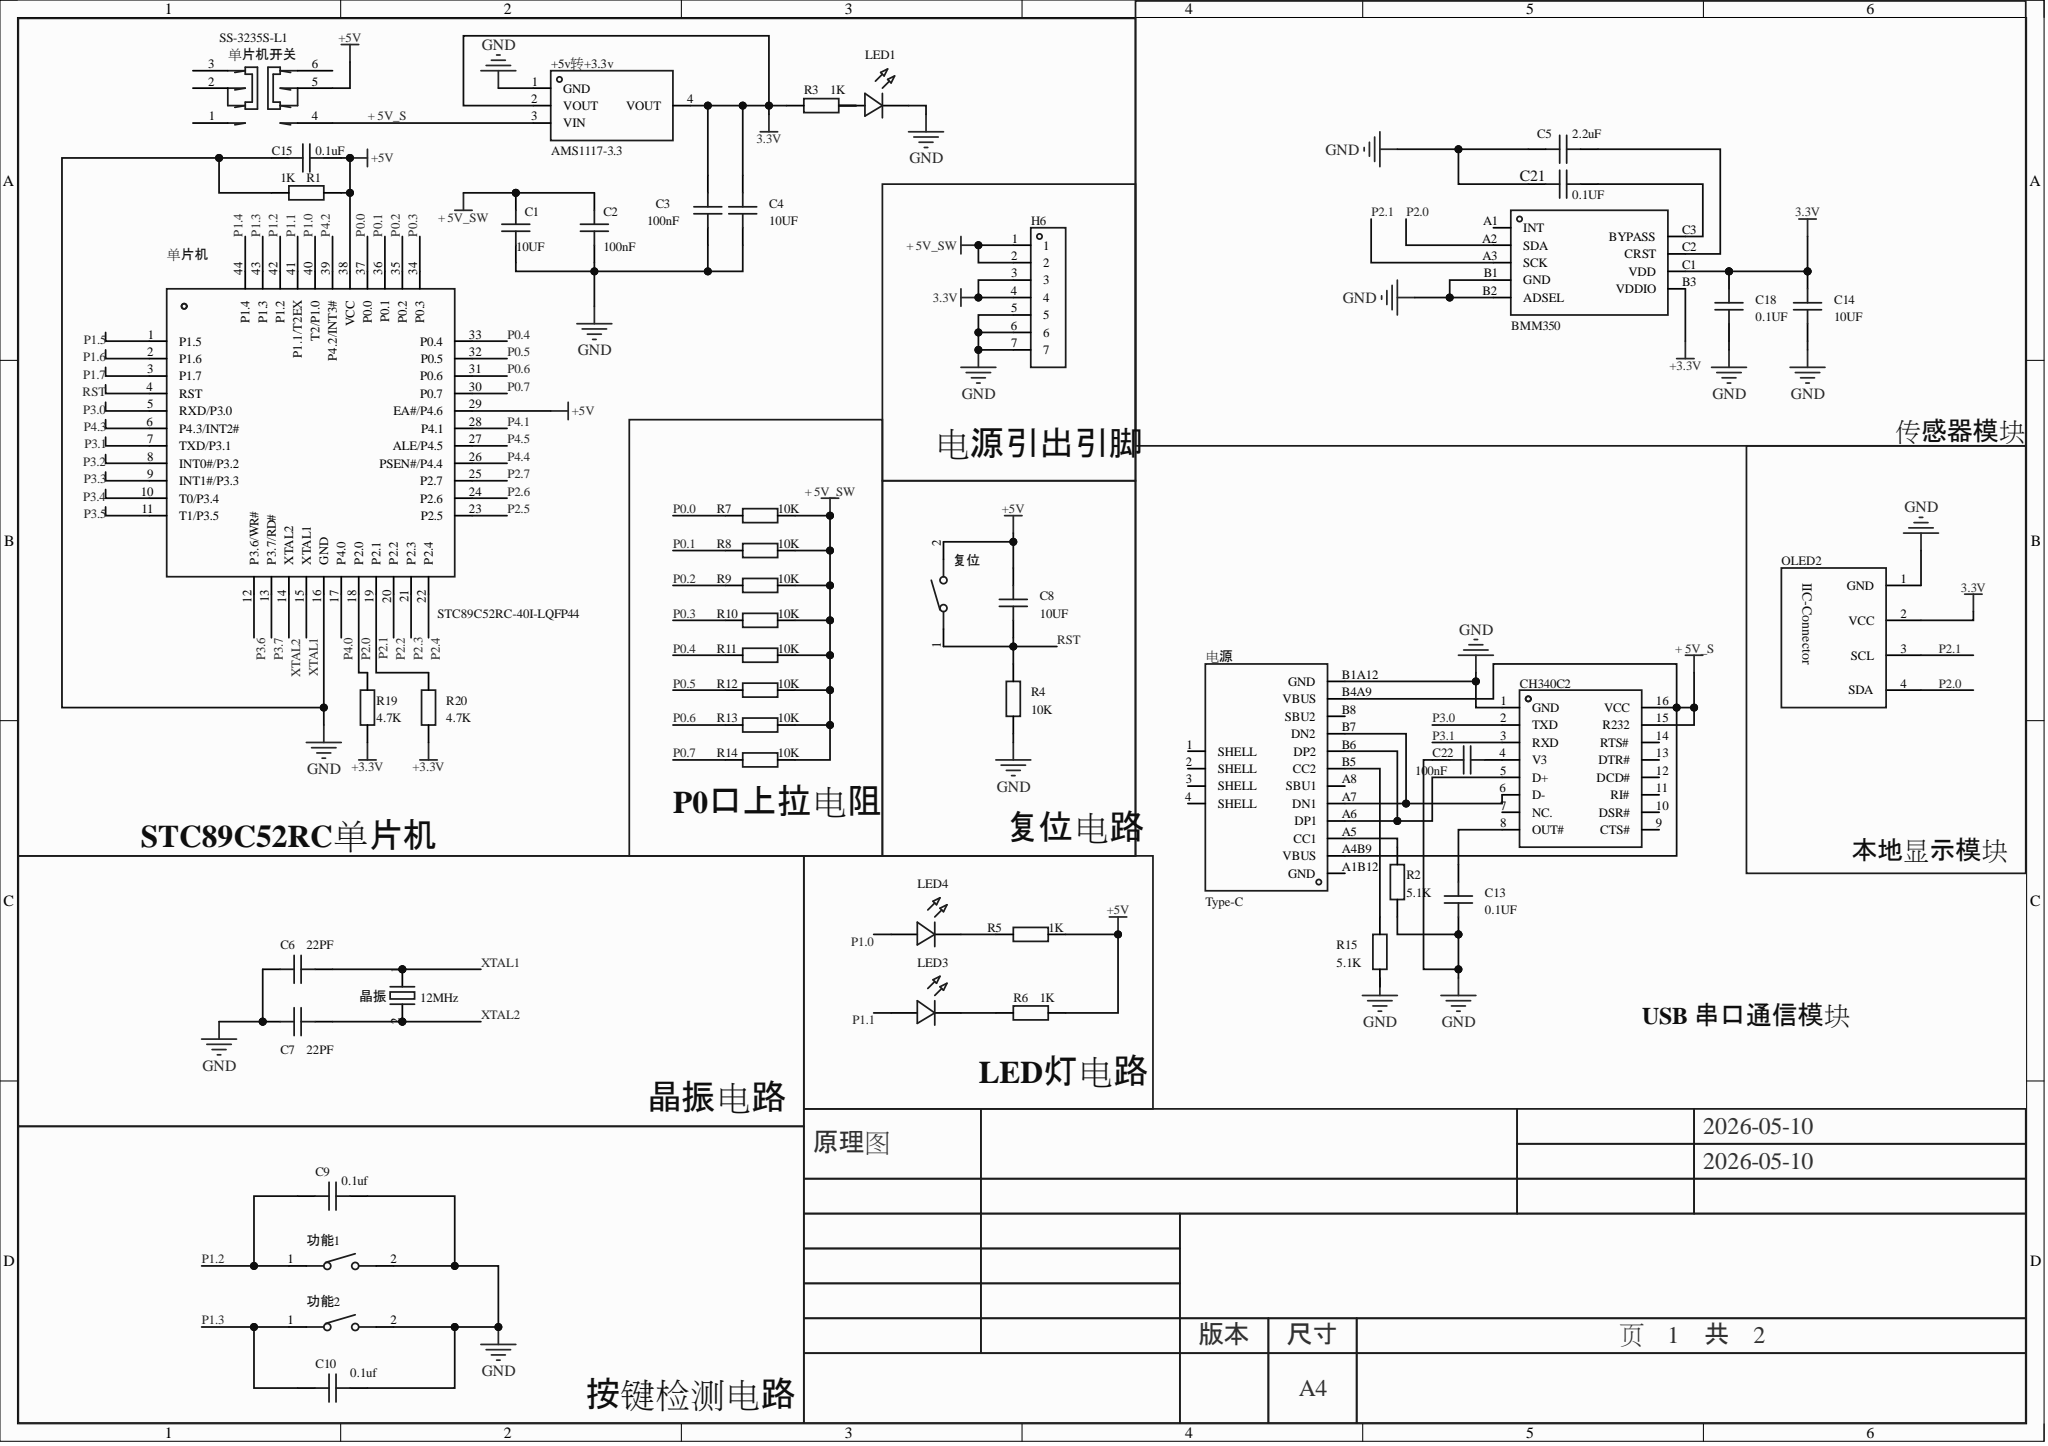Circuit board | Altium Designer | 48 parts | 34 nets
Bill of materials:
Comment,Description,Designator,Footprint,LibRef,Quantity
"AMS1117-3.3","输出类型:固定;工作电压:15V;输出电压:3.3V;输出电流:1A;电源纹波抑制比(PSRR):72dB@(120Hz);输出极性:正极;","+5v转+3.3v","SOT-223-3_L6.5-W3.4-P2.30-LS7.0-BR","AMS1117-3.3_C6186","1"
"10UF","","C1, C4, C8, C14","C0805","CAP_0805","4"
"100nF","","C2, C3","C0805","CAP_0805","2"
"2.2uF","容值:2.2uF;精度:±10%;额定电压:6.3V;材质(温度系数):X7R;","C5","C0805","CGB4B3X7R0J225K055AB","1"
"22PF","","C6, C7","C0805","CAP_0805","2"
"0.1uf","","C9, C10, C13, C15, C18, C21","C0805","CAP_0805","6"
"100nF","","C22","C0603","CAP_0603","1"
"CH340C","应用功能:收发器;USB协议版本:USB 2.0;数据速率:2Mbps;","CH340C2","SOP-16_L10.0-W3.9-P1.27-LS6.0-BL","CH340C","1"
"","","H6","HDR-TH_7P-P2.54-V-M","HDR-M_2.54_1x7P","1"
"","","LED1, LED3, LED4","LED_0805","LED_0805-G","3"
"0.96OLED_4P_MODULE_JX","","OLED2","0.96OLED_4P","0.96OLED_4P_MODULE_JX","1"
"1K","","R1, R3, R5, R6","R0805","Res_0805","4"
"5.1K","","R2, R15","R0603","Res_0603","2"
"10K","","R4, R7, R8, R9, R10, R11, R12, R13, R14","R0805","Res_0805","9"
"4.7K","","R19, R20","R0603","Res_0603","2"
"BMM350","","U1","WLCSP-9_L1.3-W1.3-R3-C3-P0.40-TL","BMM350","1"
"轻触按键3*4*H","","功能1, 功能2, 复位","SW-SMD_L4.0-W2.9-LS5.0","轻触按键3*4*H","3"
"STC89C52RC-40I-LQFP44","CPU内核:51家族;","单片机","LQFP-44_L10.0-W10.0-P0.80-LS12.0-BL","STC89C52RC-40I-LQFP44","1"
"SS-3235S-L1","电路结构:双刀双掷;安装方式:卧贴;开关颜色:黑色;额定电流:50mA;额定电压:12V;工作寿命:1万次;","单片机开关","SW-SMD_SS-3235S-LX","SS-3235S-L1","1"
"12MHz","频率:12MHz;常温频差:±30ppm;负载电容:18pF;频率稳定度:±35ppm;","晶振","CRYSTAL-SMD_L11.4-W4.7-LS12.7","ABLS-12.000MHZ-B4H-T","1"
"Type-C","","电源","USB-C-SMD_TYPE-C16PIN","Type-C-TOP_1","1"
Netlist (Protel format):
[
+5v转+3.3v
SOT-223-3_L6.5-W3.4-P2.30-LS7.0-BR
AMS1117-3.3



]
[
C1
C0805
10UF



]
[
C2
C0805
100nF



]
[
C3
C0805
100nF



]
[
C4
C0805
10UF



]
[
C5
C0805
2.2uF



]
[
C6
C0805
22PF



]
[
C7
C0805
22PF



]
[
C8
C0805
10UF



]
[
C9
C0805
0.1uf



]
[
C10
C0805
0.1uf



]
[
C13
C0805
0.1UF



]
[
C14
C0805
10UF



]
[
C15
C0805
0.1uF



]
[
C18
C0805
0.1UF



]
[
C21
C0805
0.1UF



]
[
C22
C0603
100nF



]
[
CH340C2
SOP-16_L10.0-W3.9-P1.27-LS6.0-BL
CH340C



]
[
H6
HDR-TH_7P-P2.54-V-M




]
[
LED1
LED_0805




]
[
LED3
LED_0805




]
[
LED4
LED_0805




]
[
OLED2
0.96OLED_4P
0.96OLED_4P_MODULE_JX



]
[
R1
R0805
1K



]
[
R2
R0603
5.1K



]
[
R3
R0805
1K



]
[
R4
R0805
10K



]
[
R5
R0805
1K



]
[
R6
R0805
1K



]
[
R7
R0805
10K



]
[
R8
R0805
10K



]
[
R9
R0805
10K



]
[
R10
R0805
10K



]
[
R11
R0805
10K



]
[
R12
R0805
10K



]
[
R13
R0805
10K



]
[
R14
R0805
10K



]
[
R15
R0603
5.1K



]
[
R19
R0603
4.7K



]
[
R20
R0603
4.7K



]
[
U1
WLCSP-9_L1.3-W1.3-R3-C3-P0.40-TL
BMM350



]
[
功能1
SW-SMD_L4.0-W2.9-LS5.0
轻触按键3*4*H



]
[
功能2
SW-SMD_L4.0-W2.9-LS5.0
轻触按键3*4*H



]
[
单片机
LQFP-44_L10.0-W10.0-P0.80-LS12.0-BL
STC89C52RC-40I-LQFP44



]
[
单片机开关
SW-SMD_SS-3235S-LX
SS-3235S-L1



]
[
复位
SW-SMD_L4.0-W2.9-LS5.0
轻触按键3*4*H



]
[
晶振
CRYSTAL-SMD_L11.4-W4.7-LS12.7
12MHz



]
[
电源
USB-C-SMD_TYPE-C16PIN
Type-C



]
(
XTAL2
C7-1
单片机-14
晶振-2
)
(
XTAL1
C6-1
单片机-15
晶振-1
)
(
RST
C8-2
R4-2
单片机-4
复位-1
)
(
P3.1
CH340C2-3
单片机-7
)
(
P3.0
CH340C2-2
单片机-5
)
(
P2.1
OLED2-3
R20-2
U1-A3
单片机-19
)
(
P2.0
OLED2-4
R19-2
U1-A2
单片机-18
)
(
P1.3
C10-2
功能2-1
单片机-43
)
(
P1.2
C9-2
功能1-1
单片机-42
)
(
P1.1
LED3-2
单片机-41
)
(
P1.0
LED4-2
单片机-40
)
(
P0.7
R14-1
单片机-30
)
(
P0.6
R13-1
单片机-31
)
(
P0.5
R12-1
单片机-32
)
(
P0.4
R11-1
单片机-33
)
(
P0.3
R10-1
单片机-34
)
(
P0.2
R9-1
单片机-35
)
(
P0.1
R8-1
单片机-36
)
(
P0.0
R7-1
单片机-37
)
(
NetR15_2
R15-2
电源-B5
)
(
NetR2_2
R2-2
电源-A5
)
(
NetLED4_1
LED4-1
R5-1
)
(
NetLED3_1
LED3-1
R6-1
)
(
NetLED1_2
LED1-2
R3-2
)
(
NetCH340C2_6
CH340C2-6
电源-A7
电源-B7
)
(
NetCH340C2_5
CH340C2-5
电源-A6
电源-B6
)
(
NetC22_2
C22-2
CH340C2-4
)
(
NetC21_2
C21-2
U1-C3
)
(
NetC13_2
C13-2
CH340C2-8
)
(
NetC5_1
C5-1
U1-C2
)
(
GND
+5v转+3.3v-1
C1-1
C2-1
C3-1
C4-1
C5-2
C6-2
C7-2
C9-1
C10-1
C13-1
C14-2
C15-1
C18-1
C21-1
C22-1
CH340C2-1
H6-5
H6-6
H6-7
LED1-1
OLED2-1
R1-1
R2-1
R4-1
R15-1
U1-B1
U1-B2
功能1-2
功能2-2
单片机-16
电源-B1A12
)
(
+ 5V_S
+5v转+3.3v-3
CH340C2-15
CH340C2-16
单片机开关-4
电源-A4B9
电源-B4A9
)
(
+3.3V
C1-2
C2-2
C8-1
C15-2
H6-1
H6-2
R1-2
R5-2
R6-2
R7-2
R8-2
R9-2
R10-2
R11-2
R12-2
R13-2
R14-2
R19-1
R20-1
U1-B3
单片机-29
单片机-38
单片机开关-5
复位-2
)
(
3.3V
+5v转+3.3v-2
+5v转+3.3v-4
C3-2
C4-2
C14-1
C18-2
H6-3
H6-4
OLED2-2
R3-1
U1-C1
)